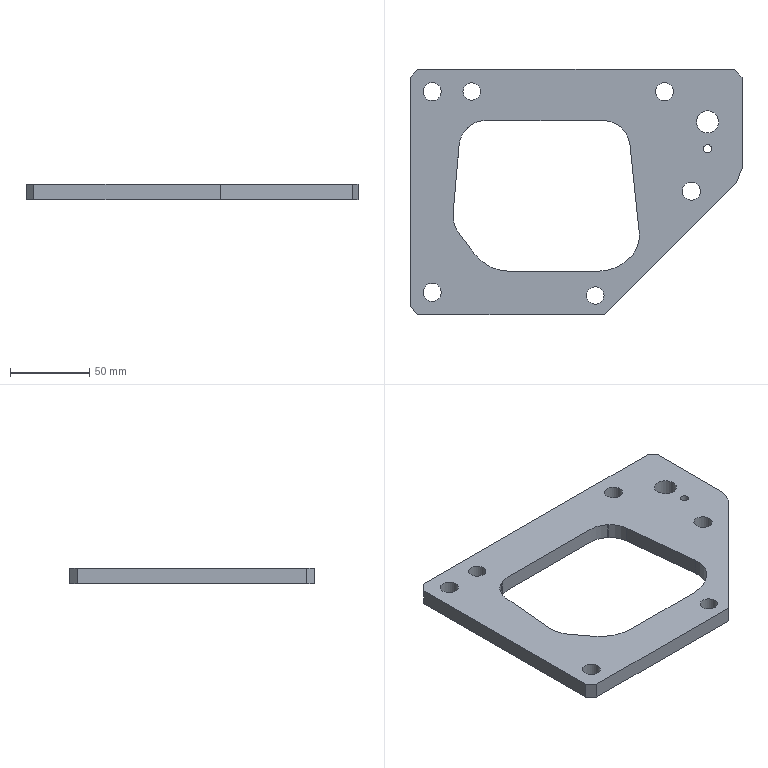Part | STEP file | lll_id510_x_t | 1 solid | 46 faces | box 210 x 155 x 10 mm | volume 176857 mm3 | spline 19 | plane 17 | cylinder 10 | commonest cylinder face diameters 11.509 x4 11 x2 5.206 x1 14 x1 38 x1 58 x1